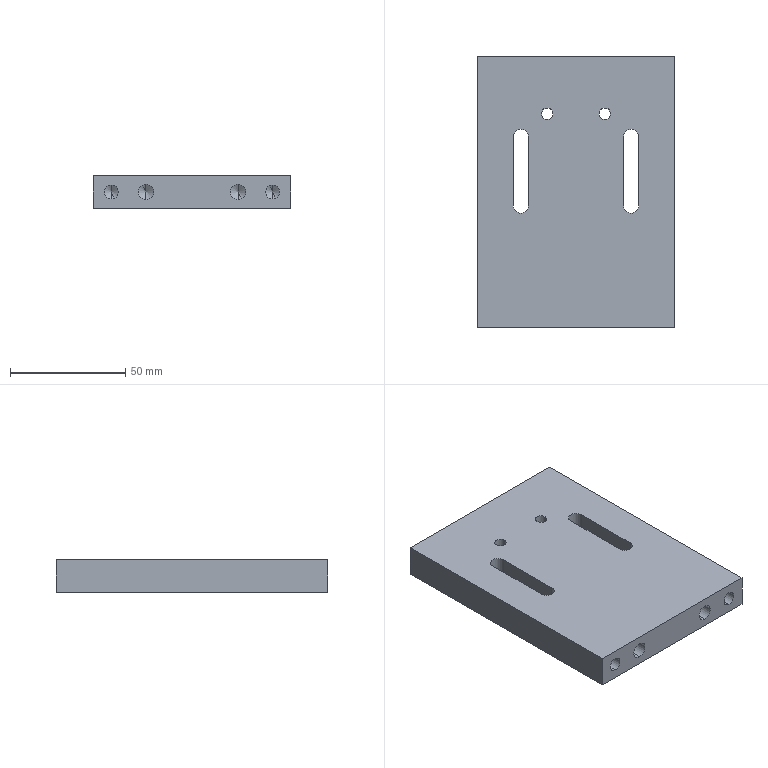Part | STEP file | 1 solid | 42 faces | box 86 x 118 x 14 mm | volume 130717 mm3 | cylinder 20 | cone 12 | plane 10 | commonest cylinder face diameters 6.8 x8 5 x4 6 x4 6.5 x4